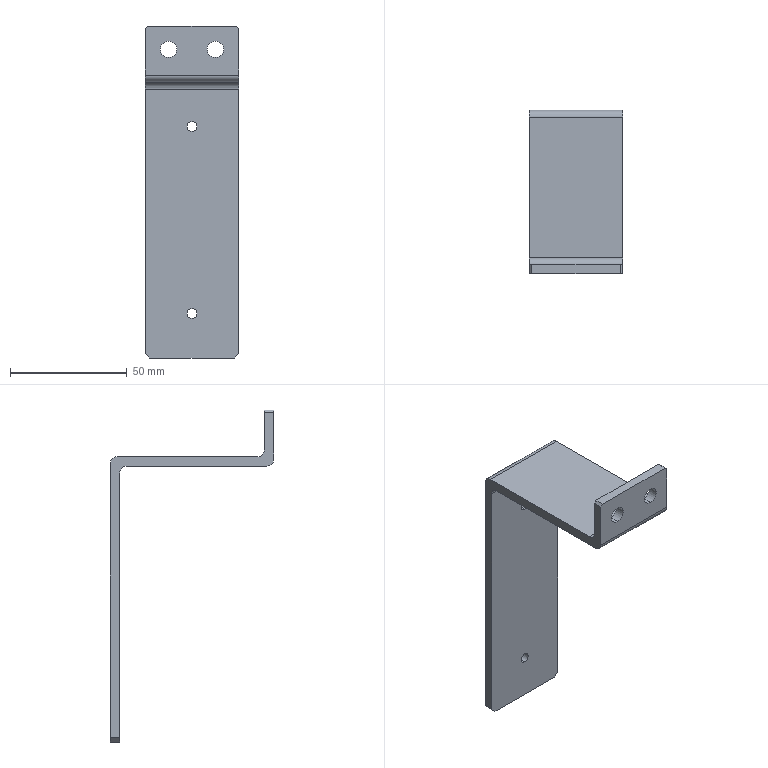Part | STEP file | Cable Carrier Channel Bracket | 1 solid | 26 faces | box 40 x 70 x 142 mm | volume 32841 mm3 | plane 14 | cylinder 12 | commonest cylinder face diameters 4.2 x4 6 x4 7 x4